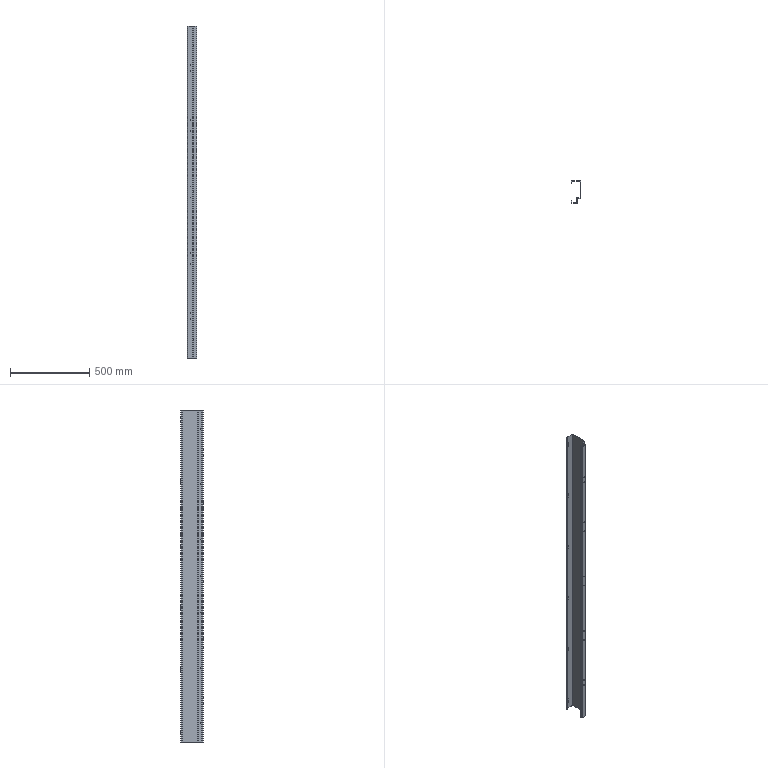Part | SolidWorks | features ICE 3, FlatPattern 1, MirrorPattern 1, SMBaseFlange 1, SheetMetal 1 | 1 solid | 118 faces | box 58 x 140 x 2100 mm | volume 680862 mm3 | cylinder 64 | plane 54 | commonest cylinder face diameters 5 x20 9 x18 4.6 x14 2 x6 4.4 x6